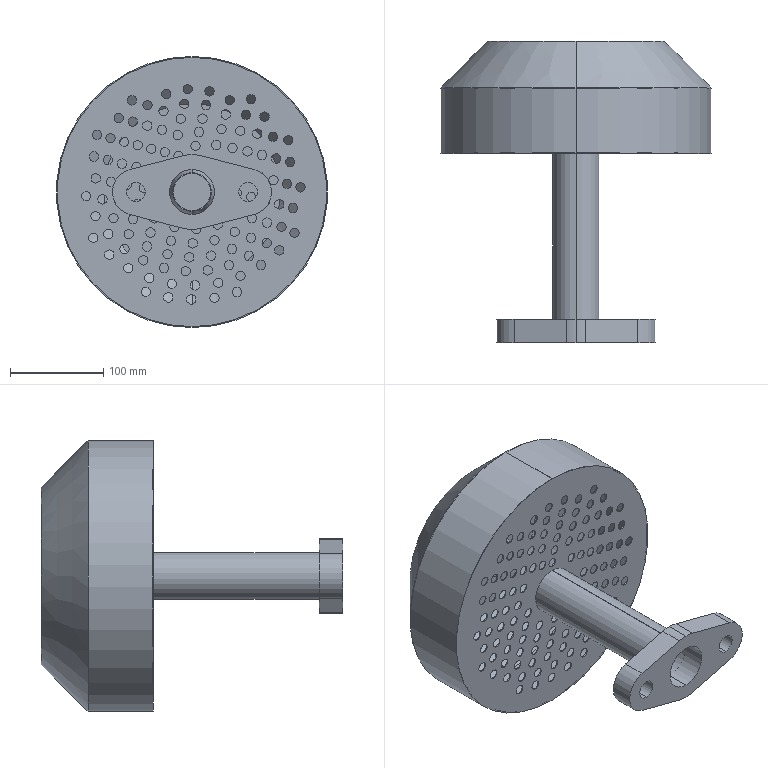Part | SolidWorks | 1 solid | 267 faces | box 290 x 322.5 x 290 mm | volume 420186 mm3 | cylinder 247 | plane 12 | cone 8 | commonest cylinder face diameters 10 x230 20 x4 50 x4 80 x3 48 x2 288 x2